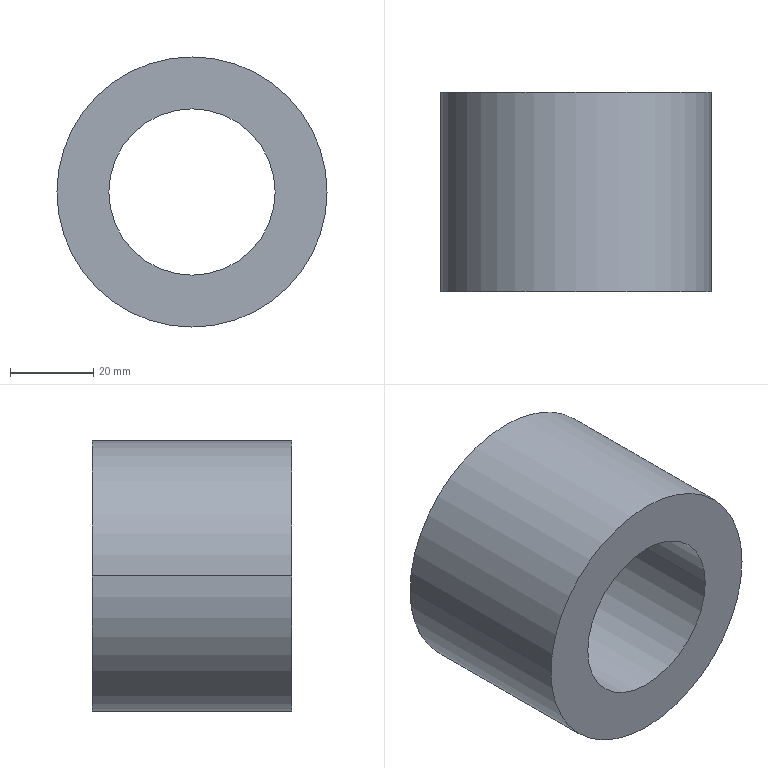Part | STEP file | PN_0061_default | 1 solid | 6 faces | box 65 x 48 x 65 mm | volume 98960 mm3 | cylinder 4 | plane 2 | commonest cylinder face diameters 40 x2 65 x2
STEP:
#1=CARTESIAN_POINT('',(0.,0.,0.));
#2=DIRECTION('',(0.,0.,1.));
#3=DIRECTION('',(1.,0.,0.));
#4=AXIS2_PLACEMENT_3D('',#1,#2,#3);
#5=CARTESIAN_POINT('',(20.,-24.,0.));
#6=VERTEX_POINT('',#5);
#7=CARTESIAN_POINT('',(-20.,-24.,0.));
#8=VERTEX_POINT('',#7);
#9=CARTESIAN_POINT('',(0.,-24.,0.));
#10=DIRECTION('',(0.,1.,0.));
#11=DIRECTION('',(1.,0.,0.));
#12=AXIS2_PLACEMENT_3D('',#9,#10,#11);
#13=CIRCLE('',#12,20.);
#14=CARTESIAN_POINT('',(2.522,-24.,0.));
#15=DIRECTION('',(0.,1.,0.));
#16=DIRECTION('',(1.,0.,0.));
#17=AXIS2_PLACEMENT_3D('',#14,#15,#16);
#18=PLANE('',#17);
#19=CARTESIAN_POINT('',(-2.522,0.));
#20=DIRECTION('',(1.,0.));
#21=AXIS2_PLACEMENT_2D('',#19,#20);
#22=CIRCLE('',#21,20.);
#23=(GEOMETRIC_REPRESENTATION_CONTEXT(2)PARAMETRIC_REPRESENTATION_CONTEXT()REPRESENTATION_CONTEXT('',''));
#24=DEFINITIONAL_REPRESENTATION('',(#22),#23);
#25=PCURVE('',#18,#24);
#26=CARTESIAN_POINT('',(0.,-24.,0.));
#27=DIRECTION('',(0.,1.,0.));
#28=DIRECTION('',(1.,0.,0.));
#29=AXIS2_PLACEMENT_3D('',#26,#27,#28);
#30=CYLINDRICAL_SURFACE('',#29,20.);
#31=CARTESIAN_POINT('',(0.,0.));
#32=DIRECTION('',(1.,0.));
#33=VECTOR('',#32,1.);
#34=LINE('',#31,#33);
#35=(GEOMETRIC_REPRESENTATION_CONTEXT(2)PARAMETRIC_REPRESENTATION_CONTEXT()REPRESENTATION_CONTEXT('',''));
#36=DEFINITIONAL_REPRESENTATION('',(#34),#35);
#37=PCURVE('',#30,#36);
#38=SURFACE_CURVE('',#13,(#25,#37),.PCURVE_S1.);
#39=EDGE_CURVE('',#6,#8,#38,.T.);
#40=ORIENTED_EDGE('',*,*,#39,.T.);
#41=CARTESIAN_POINT('',(0.,-24.,0.));
#42=DIRECTION('',(0.,1.,0.));
#43=DIRECTION('',(1.,0.,0.));
#44=AXIS2_PLACEMENT_3D('',#41,#42,#43);
#45=CIRCLE('',#44,20.);
#46=CARTESIAN_POINT('',(-2.522,0.));
#47=DIRECTION('',(1.,0.));
#48=AXIS2_PLACEMENT_2D('',#46,#47);
#49=CIRCLE('',#48,20.);
#50=(GEOMETRIC_REPRESENTATION_CONTEXT(2)PARAMETRIC_REPRESENTATION_CONTEXT()REPRESENTATION_CONTEXT('',''));
#51=DEFINITIONAL_REPRESENTATION('',(#49),#50);
#52=PCURVE('',#18,#51);
#53=CARTESIAN_POINT('',(0.,-24.,0.));
#54=DIRECTION('',(0.,1.,0.));
#55=DIRECTION('',(1.,0.,0.));
#56=AXIS2_PLACEMENT_3D('',#53,#54,#55);
#57=CYLINDRICAL_SURFACE('',#56,20.);
#58=CARTESIAN_POINT('',(0.,0.));
#59=DIRECTION('',(1.,0.));
#60=VECTOR('',#59,1.);
#61=LINE('',#58,#60);
#62=(GEOMETRIC_REPRESENTATION_CONTEXT(2)PARAMETRIC_REPRESENTATION_CONTEXT()REPRESENTATION_CONTEXT('',''));
#63=DEFINITIONAL_REPRESENTATION('',(#61),#62);
#64=PCURVE('',#57,#63);
#65=SURFACE_CURVE('',#45,(#52,#64),.PCURVE_S1.);
#66=EDGE_CURVE('',#8,#6,#65,.T.);
#67=ORIENTED_EDGE('',*,*,#66,.T.);
#68=EDGE_LOOP('',(#40,#67));
#69=FACE_BOUND('',#68,.T.);
#70=CARTESIAN_POINT('',(32.5,-24.,0.));
#71=VERTEX_POINT('',#70);
#72=CARTESIAN_POINT('',(-32.5,-24.,0.));
#73=VERTEX_POINT('',#72);
#74=CARTESIAN_POINT('',(0.,-24.,0.));
#75=DIRECTION('',(0.,-1.,0.));
#76=DIRECTION('',(1.,0.,0.));
#77=AXIS2_PLACEMENT_3D('',#74,#75,#76);
#78=CIRCLE('',#77,32.5);
#79=CARTESIAN_POINT('',(29.978,0.));
#80=CARTESIAN_POINT('',(29.978,-56.292));
#81=CARTESIAN_POINT('',(-18.772,-28.146));
#82=CARTESIAN_POINT('',(-67.522,0.));
#83=CARTESIAN_POINT('',(-18.772,28.146));
#84=CARTESIAN_POINT('',(29.978,56.292));
#85=CARTESIAN_POINT('',(29.978,0.));
#86=(BOUNDED_CURVE()B_SPLINE_CURVE(2,(#79,#80,#81,#82,#83,#84,#85),.UNSPECIFIED.,.T.,.F.)B_SPLINE_CURVE_WITH_KNOTS((1,2,2,2,2,1),(-2.094,0.,2.094,4.189,6.283,8.378),.UNSPECIFIED.)CURVE()GEOMETRIC_REPRESENTATION_ITEM()RATIONAL_B_SPLINE_CURVE((1.,0.5,1.,0.5,1.,0.5,1.))REPRESENTATION_ITEM(''));
#87=(GEOMETRIC_REPRESENTATION_CONTEXT(2)PARAMETRIC_REPRESENTATION_CONTEXT()REPRESENTATION_CONTEXT('',''));
#88=DEFINITIONAL_REPRESENTATION('',(#86),#87);
#89=PCURVE('',#18,#88);
#90=CARTESIAN_POINT('',(0.,-24.,0.));
#91=DIRECTION('',(0.,1.,0.));
#92=DIRECTION('',(1.,0.,0.));
#93=AXIS2_PLACEMENT_3D('',#90,#91,#92);
#94=CYLINDRICAL_SURFACE('',#93,32.5);
#95=CARTESIAN_POINT('',(6.283,0.));
#96=DIRECTION('',(-1.,0.));
#97=VECTOR('',#96,1.);
#98=LINE('',#95,#97);
#99=(GEOMETRIC_REPRESENTATION_CONTEXT(2)PARAMETRIC_REPRESENTATION_CONTEXT()REPRESENTATION_CONTEXT('',''));
#100=DEFINITIONAL_REPRESENTATION('',(#98),#99);
#101=PCURVE('',#94,#100);
#102=SURFACE_CURVE('',#78,(#89,#101),.PCURVE_S1.);
#103=EDGE_CURVE('',#71,#73,#102,.T.);
#104=ORIENTED_EDGE('',*,*,#103,.T.);
#105=CARTESIAN_POINT('',(0.,-24.,0.));
#106=DIRECTION('',(0.,-1.,0.));
#107=DIRECTION('',(1.,0.,0.));
#108=AXIS2_PLACEMENT_3D('',#105,#106,#107);
#109=CIRCLE('',#108,32.5);
#110=CARTESIAN_POINT('',(29.978,0.));
#111=CARTESIAN_POINT('',(29.978,-56.292));
#112=CARTESIAN_POINT('',(-18.772,-28.146));
#113=CARTESIAN_POINT('',(-67.522,0.));
#114=CARTESIAN_POINT('',(-18.772,28.146));
#115=CARTESIAN_POINT('',(29.978,56.292));
#116=CARTESIAN_POINT('',(29.978,0.));
#117=(BOUNDED_CURVE()B_SPLINE_CURVE(2,(#110,#111,#112,#113,#114,#115,#116),.UNSPECIFIED.,.T.,.F.)B_SPLINE_CURVE_WITH_KNOTS((1,2,2,2,2,1),(-2.094,0.,2.094,4.189,6.283,8.378),.UNSPECIFIED.)CURVE()GEOMETRIC_REPRESENTATION_ITEM()RATIONAL_B_SPLINE_CURVE((1.,0.5,1.,0.5,1.,0.5,1.))REPRESENTATION_ITEM(''));
#118=(GEOMETRIC_REPRESENTATION_CONTEXT(2)PARAMETRIC_REPRESENTATION_CONTEXT()REPRESENTATION_CONTEXT('',''));
#119=DEFINITIONAL_REPRESENTATION('',(#117),#118);
#120=PCURVE('',#18,#119);
#121=CARTESIAN_POINT('',(0.,-24.,0.));
#122=DIRECTION('',(0.,1.,0.));
#123=DIRECTION('',(1.,0.,0.));
#124=AXIS2_PLACEMENT_3D('',#121,#122,#123);
#125=CYLINDRICAL_SURFACE('',#124,32.5);
#126=CARTESIAN_POINT('',(6.283,0.));
#127=DIRECTION('',(-1.,0.));
#128=VECTOR('',#127,1.);
#129=LINE('',#126,#128);
#130=(GEOMETRIC_REPRESENTATION_CONTEXT(2)PARAMETRIC_REPRESENTATION_CONTEXT()REPRESENTATION_CONTEXT('',''));
#131=DEFINITIONAL_REPRESENTATION('',(#129),#130);
#132=PCURVE('',#125,#131);
#133=SURFACE_CURVE('',#109,(#120,#132),.PCURVE_S1.);
#134=EDGE_CURVE('',#73,#71,#133,.T.);
#135=ORIENTED_EDGE('',*,*,#134,.T.);
#136=EDGE_LOOP('',(#104,#135));
#137=FACE_BOUND('',#136,.T.);
#138=ADVANCED_FACE('',(#69,#137),#18,.F.);
#139=CARTESIAN_POINT('',(20.,24.,0.));
#140=VERTEX_POINT('',#139);
#141=CARTESIAN_POINT('',(-20.,24.,0.));
#142=VERTEX_POINT('',#141);
#143=CARTESIAN_POINT('',(0.,24.,0.));
#144=DIRECTION('',(0.,1.,0.));
#145=DIRECTION('',(1.,0.,0.));
#146=AXIS2_PLACEMENT_3D('',#143,#144,#145);
#147=CIRCLE('',#146,20.);
#148=CARTESIAN_POINT('',(2.522,24.,0.));
#149=DIRECTION('',(0.,1.,0.));
#150=DIRECTION('',(1.,0.,0.));
#151=AXIS2_PLACEMENT_3D('',#148,#149,#150);
#152=PLANE('',#151);
#153=CARTESIAN_POINT('',(-2.522,0.));
#154=DIRECTION('',(1.,0.));
#155=AXIS2_PLACEMENT_2D('',#153,#154);
#156=CIRCLE('',#155,20.);
#157=(GEOMETRIC_REPRESENTATION_CONTEXT(2)PARAMETRIC_REPRESENTATION_CONTEXT()REPRESENTATION_CONTEXT('',''));
#158=DEFINITIONAL_REPRESENTATION('',(#156),#157);
#159=PCURVE('',#152,#158);
#160=CARTESIAN_POINT('',(0.,48.));
#161=DIRECTION('',(1.,0.));
#162=VECTOR('',#161,1.);
#163=LINE('',#160,#162);
#164=(GEOMETRIC_REPRESENTATION_CONTEXT(2)PARAMETRIC_REPRESENTATION_CONTEXT()REPRESENTATION_CONTEXT('',''));
#165=DEFINITIONAL_REPRESENTATION('',(#163),#164);
#166=PCURVE('',#30,#165);
#167=SURFACE_CURVE('',#147,(#159,#166),.PCURVE_S1.);
#168=EDGE_CURVE('',#140,#142,#167,.T.);
#169=ORIENTED_EDGE('',*,*,#168,.F.);
#170=CARTESIAN_POINT('',(0.,24.,0.));
#171=DIRECTION('',(0.,1.,0.));
#172=DIRECTION('',(1.,0.,0.));
#173=AXIS2_PLACEMENT_3D('',#170,#171,#172);
#174=CIRCLE('',#173,20.);
#175=CARTESIAN_POINT('',(-2.522,0.));
#176=DIRECTION('',(1.,0.));
#177=AXIS2_PLACEMENT_2D('',#175,#176);
#178=CIRCLE('',#177,20.);
#179=(GEOMETRIC_REPRESENTATION_CONTEXT(2)PARAMETRIC_REPRESENTATION_CONTEXT()REPRESENTATION_CONTEXT('',''));
#180=DEFINITIONAL_REPRESENTATION('',(#178),#179);
#181=PCURVE('',#152,#180);
#182=CARTESIAN_POINT('',(0.,48.));
#183=DIRECTION('',(1.,0.));
#184=VECTOR('',#183,1.);
#185=LINE('',#182,#184);
#186=(GEOMETRIC_REPRESENTATION_CONTEXT(2)PARAMETRIC_REPRESENTATION_CONTEXT()REPRESENTATION_CONTEXT('',''));
#187=DEFINITIONAL_REPRESENTATION('',(#185),#186);
#188=PCURVE('',#57,#187);
#189=SURFACE_CURVE('',#174,(#181,#188),.PCURVE_S1.);
#190=EDGE_CURVE('',#142,#140,#189,.T.);
#191=ORIENTED_EDGE('',*,*,#190,.F.);
#192=EDGE_LOOP('',(#169,#191));
#193=FACE_BOUND('',#192,.T.);
#194=CARTESIAN_POINT('',(32.5,24.,0.));
#195=VERTEX_POINT('',#194);
#196=CARTESIAN_POINT('',(-32.5,24.,0.));
#197=VERTEX_POINT('',#196);
#198=CARTESIAN_POINT('',(0.,24.,0.));
#199=DIRECTION('',(0.,-1.,0.));
#200=DIRECTION('',(1.,0.,0.));
#201=AXIS2_PLACEMENT_3D('',#198,#199,#200);
#202=CIRCLE('',#201,32.5);
#203=CARTESIAN_POINT('',(29.978,0.));
#204=CARTESIAN_POINT('',(29.978,-56.292));
#205=CARTESIAN_POINT('',(-18.772,-28.146));
#206=CARTESIAN_POINT('',(-67.522,0.));
#207=CARTESIAN_POINT('',(-18.772,28.146));
#208=CARTESIAN_POINT('',(29.978,56.292));
#209=CARTESIAN_POINT('',(29.978,0.));
#210=(BOUNDED_CURVE()B_SPLINE_CURVE(2,(#203,#204,#205,#206,#207,#208,#209),.UNSPECIFIED.,.T.,.F.)B_SPLINE_CURVE_WITH_KNOTS((1,2,2,2,2,1),(-2.094,0.,2.094,4.189,6.283,8.378),.UNSPECIFIED.)CURVE()GEOMETRIC_REPRESENTATION_ITEM()RATIONAL_B_SPLINE_CURVE((1.,0.5,1.,0.5,1.,0.5,1.))REPRESENTATION_ITEM(''));
#211=(GEOMETRIC_REPRESENTATION_CONTEXT(2)PARAMETRIC_REPRESENTATION_CONTEXT()REPRESENTATION_CONTEXT('',''));
#212=DEFINITIONAL_REPRESENTATION('',(#210),#211);
#213=PCURVE('',#152,#212);
#214=CARTESIAN_POINT('',(6.283,48.));
#215=DIRECTION('',(-1.,0.));
#216=VECTOR('',#215,1.);
#217=LINE('',#214,#216);
#218=(GEOMETRIC_REPRESENTATION_CONTEXT(2)PARAMETRIC_REPRESENTATION_CONTEXT()REPRESENTATION_CONTEXT('',''));
#219=DEFINITIONAL_REPRESENTATION('',(#217),#218);
#220=PCURVE('',#94,#219);
#221=SURFACE_CURVE('',#202,(#213,#220),.PCURVE_S1.);
#222=EDGE_CURVE('',#195,#197,#221,.T.);
#223=ORIENTED_EDGE('',*,*,#222,.F.);
#224=CARTESIAN_POINT('',(0.,24.,0.));
#225=DIRECTION('',(0.,-1.,0.));
#226=DIRECTION('',(1.,0.,0.));
#227=AXIS2_PLACEMENT_3D('',#224,#225,#226);
#228=CIRCLE('',#227,32.5);
#229=CARTESIAN_POINT('',(29.978,0.));
#230=CARTESIAN_POINT('',(29.978,-56.292));
#231=CARTESIAN_POINT('',(-18.772,-28.146));
#232=CARTESIAN_POINT('',(-67.522,0.));
#233=CARTESIAN_POINT('',(-18.772,28.146));
#234=CARTESIAN_POINT('',(29.978,56.292));
#235=CARTESIAN_POINT('',(29.978,0.));
#236=(BOUNDED_CURVE()B_SPLINE_CURVE(2,(#229,#230,#231,#232,#233,#234,#235),.UNSPECIFIED.,.T.,.F.)B_SPLINE_CURVE_WITH_KNOTS((1,2,2,2,2,1),(-2.094,0.,2.094,4.189,6.283,8.378),.UNSPECIFIED.)CURVE()GEOMETRIC_REPRESENTATION_ITEM()RATIONAL_B_SPLINE_CURVE((1.,0.5,1.,0.5,1.,0.5,1.))REPRESENTATION_ITEM(''));
#237=(GEOMETRIC_REPRESENTATION_CONTEXT(2)PARAMETRIC_REPRESENTATION_CONTEXT()REPRESENTATION_CONTEXT('',''));
#238=DEFINITIONAL_REPRESENTATION('',(#236),#237);
#239=PCURVE('',#152,#238);
#240=CARTESIAN_POINT('',(6.283,48.));
#241=DIRECTION('',(-1.,0.));
#242=VECTOR('',#241,1.);
#243=LINE('',#240,#242);
#244=(GEOMETRIC_REPRESENTATION_CONTEXT(2)PARAMETRIC_REPRESENTATION_CONTEXT()REPRESENTATION_CONTEXT('',''));
#245=DEFINITIONAL_REPRESENTATION('',(#243),#244);
#246=PCURVE('',#125,#245);
#247=SURFACE_CURVE('',#228,(#239,#246),.PCURVE_S1.);
#248=EDGE_CURVE('',#197,#195,#247,.T.);
#249=ORIENTED_EDGE('',*,*,#248,.F.);
#250=EDGE_LOOP('',(#223,#249));
#251=FACE_BOUND('',#250,.T.);
#252=ADVANCED_FACE('',(#193,#251),#152,.T.);
#253=ORIENTED_EDGE('',*,*,#190,.F.);
#254=CARTESIAN_POINT('',(-20.,24.,0.));
#255=DIRECTION('',(0.,-1.,0.));
#256=VECTOR('',#255,1.);
#257=LINE('',#254,#256);
#258=CARTESIAN_POINT('',(3.142,48.));
#259=DIRECTION('',(0.,-1.));
#260=VECTOR('',#259,1.);
#261=LINE('',#258,#260);
#262=(GEOMETRIC_REPRESENTATION_CONTEXT(2)PARAMETRIC_REPRESENTATION_CONTEXT()REPRESENTATION_CONTEXT('',''));
#263=DEFINITIONAL_REPRESENTATION('',(#261),#262);
#264=PCURVE('',#57,#263);
#265=CARTESIAN_POINT('',(3.142,48.));
#266=DIRECTION('',(0.,-1.));
#267=VECTOR('',#266,1.);
#268=LINE('',#265,#267);
#269=(GEOMETRIC_REPRESENTATION_CONTEXT(2)PARAMETRIC_REPRESENTATION_CONTEXT()REPRESENTATION_CONTEXT('',''));
#270=DEFINITIONAL_REPRESENTATION('',(#268),#269);
#271=PCURVE('',#30,#270);
#272=SURFACE_CURVE('',#257,(#264,#271),.PCURVE_S1.);
#273=EDGE_CURVE('',#142,#8,#272,.T.);
#274=ORIENTED_EDGE('',*,*,#273,.T.);
#275=ORIENTED_EDGE('',*,*,#66,.T.);
#276=CARTESIAN_POINT('',(20.,24.,0.));
#277=DIRECTION('',(0.,-1.,0.));
#278=VECTOR('',#277,1.);
#279=LINE('',#276,#278);
#280=CARTESIAN_POINT('',(6.283,48.));
#281=DIRECTION('',(0.,-1.));
#282=VECTOR('',#281,1.);
#283=LINE('',#280,#282);
#284=(GEOMETRIC_REPRESENTATION_CONTEXT(2)PARAMETRIC_REPRESENTATION_CONTEXT()REPRESENTATION_CONTEXT('',''));
#285=DEFINITIONAL_REPRESENTATION('',(#283),#284);
#286=PCURVE('',#57,#285);
#287=CARTESIAN_POINT('',(0.,48.));
#288=DIRECTION('',(0.,-1.));
#289=VECTOR('',#288,1.);
#290=LINE('',#287,#289);
#291=(GEOMETRIC_REPRESENTATION_CONTEXT(2)PARAMETRIC_REPRESENTATION_CONTEXT()REPRESENTATION_CONTEXT('',''));
#292=DEFINITIONAL_REPRESENTATION('',(#290),#291);
#293=PCURVE('',#30,#292);
#294=SURFACE_CURVE('',#279,(#286,#293),.PCURVE_S1.);
#295=EDGE_CURVE('',#140,#6,#294,.T.);
#296=ORIENTED_EDGE('',*,*,#295,.F.);
#297=EDGE_LOOP('',(#253,#274,#275,#296));
#298=FACE_BOUND('',#297,.F.);
#299=ADVANCED_FACE('',(#298),#57,.F.);
#300=CARTESIAN_POINT('',(32.5,24.,0.));
#301=DIRECTION('',(0.,-1.,0.));
#302=VECTOR('',#301,1.);
#303=LINE('',#300,#302);
#304=CARTESIAN_POINT('',(0.,48.));
#305=DIRECTION('',(0.,-1.));
#306=VECTOR('',#305,1.);
#307=LINE('',#304,#306);
#308=(GEOMETRIC_REPRESENTATION_CONTEXT(2)PARAMETRIC_REPRESENTATION_CONTEXT()REPRESENTATION_CONTEXT('',''));
#309=DEFINITIONAL_REPRESENTATION('',(#307),#308);
#310=PCURVE('',#125,#309);
#311=CARTESIAN_POINT('',(6.283,48.));
#312=DIRECTION('',(0.,-1.));
#313=VECTOR('',#312,1.);
#314=LINE('',#311,#313);
#315=(GEOMETRIC_REPRESENTATION_CONTEXT(2)PARAMETRIC_REPRESENTATION_CONTEXT()REPRESENTATION_CONTEXT('',''));
#316=DEFINITIONAL_REPRESENTATION('',(#314),#315);
#317=PCURVE('',#94,#316);
#318=SURFACE_CURVE('',#303,(#310,#317),.PCURVE_S1.);
#319=EDGE_CURVE('',#195,#71,#318,.T.);
#320=ORIENTED_EDGE('',*,*,#319,.T.);
#321=ORIENTED_EDGE('',*,*,#134,.F.);
#322=CARTESIAN_POINT('',(-32.5,24.,0.));
#323=DIRECTION('',(0.,-1.,0.));
#324=VECTOR('',#323,1.);
#325=LINE('',#322,#324);
#326=CARTESIAN_POINT('',(3.142,48.));
#327=DIRECTION('',(0.,-1.));
#328=VECTOR('',#327,1.);
#329=LINE('',#326,#328);
#330=(GEOMETRIC_REPRESENTATION_CONTEXT(2)PARAMETRIC_REPRESENTATION_CONTEXT()REPRESENTATION_CONTEXT('',''));
#331=DEFINITIONAL_REPRESENTATION('',(#329),#330);
#332=PCURVE('',#125,#331);
#333=CARTESIAN_POINT('',(3.142,48.));
#334=DIRECTION('',(0.,-1.));
#335=VECTOR('',#334,1.);
#336=LINE('',#333,#335);
#337=(GEOMETRIC_REPRESENTATION_CONTEXT(2)PARAMETRIC_REPRESENTATION_CONTEXT()REPRESENTATION_CONTEXT('',''));
#338=DEFINITIONAL_REPRESENTATION('',(#336),#337);
#339=PCURVE('',#94,#338);
#340=SURFACE_CURVE('',#325,(#332,#339),.PCURVE_S1.);
#341=EDGE_CURVE('',#197,#73,#340,.T.);
#342=ORIENTED_EDGE('',*,*,#341,.F.);
#343=ORIENTED_EDGE('',*,*,#248,.T.);
#344=EDGE_LOOP('',(#320,#321,#342,#343));
#345=FACE_BOUND('',#344,.T.);
#346=ADVANCED_FACE('',(#345),#125,.T.);
#347=ORIENTED_EDGE('',*,*,#319,.F.);
#348=ORIENTED_EDGE('',*,*,#222,.T.);
#349=ORIENTED_EDGE('',*,*,#341,.T.);
#350=ORIENTED_EDGE('',*,*,#103,.F.);
#351=EDGE_LOOP('',(#347,#348,#349,#350));
#352=FACE_BOUND('',#351,.T.);
#353=ADVANCED_FACE('',(#352),#94,.T.);
#354=ORIENTED_EDGE('',*,*,#39,.T.);
#355=ORIENTED_EDGE('',*,*,#273,.F.);
#356=ORIENTED_EDGE('',*,*,#168,.F.);
#357=ORIENTED_EDGE('',*,*,#295,.T.);
#358=EDGE_LOOP('',(#354,#355,#356,#357));
#359=FACE_BOUND('',#358,.F.);
#360=ADVANCED_FACE('',(#359),#30,.F.);
#361=CLOSED_SHELL('',(#138,#252,#299,#346,#353,#360));
#362=MANIFOLD_SOLID_BREP('',#361);
#363=(LENGTH_UNIT()NAMED_UNIT(*)SI_UNIT(.MILLI.,.METRE.));
#364=UNCERTAINTY_MEASURE_WITH_UNIT(LENGTH_MEASURE(0.0000001),#363,'','');
#365=(NAMED_UNIT(*)PLANE_ANGLE_UNIT()SI_UNIT($,.RADIAN.));
#366=(NAMED_UNIT(*)SI_UNIT($,.STERADIAN.)SOLID_ANGLE_UNIT());
#367=(GEOMETRIC_REPRESENTATION_CONTEXT(3)GLOBAL_UNCERTAINTY_ASSIGNED_CONTEXT((#364))GLOBAL_UNIT_ASSIGNED_CONTEXT((#363,#365,#366))REPRESENTATION_CONTEXT('',''));
#368=ADVANCED_BREP_SHAPE_REPRESENTATION('',(#4,#362),#367);